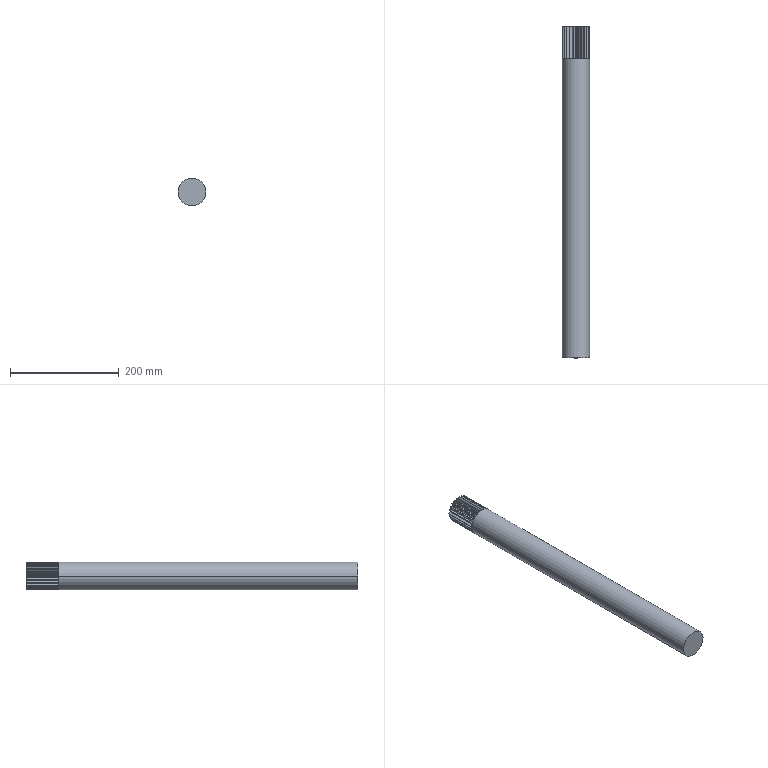Part | SolidWorks | features ICE 1, MBimport 1 | 1 solid | 98 faces | box 51 x 611.661 x 51 mm | volume 1227372 mm3 | spline 69 | cylinder 26 | plane 3 | commonest cylinder face diameters 43 x24 51 x2